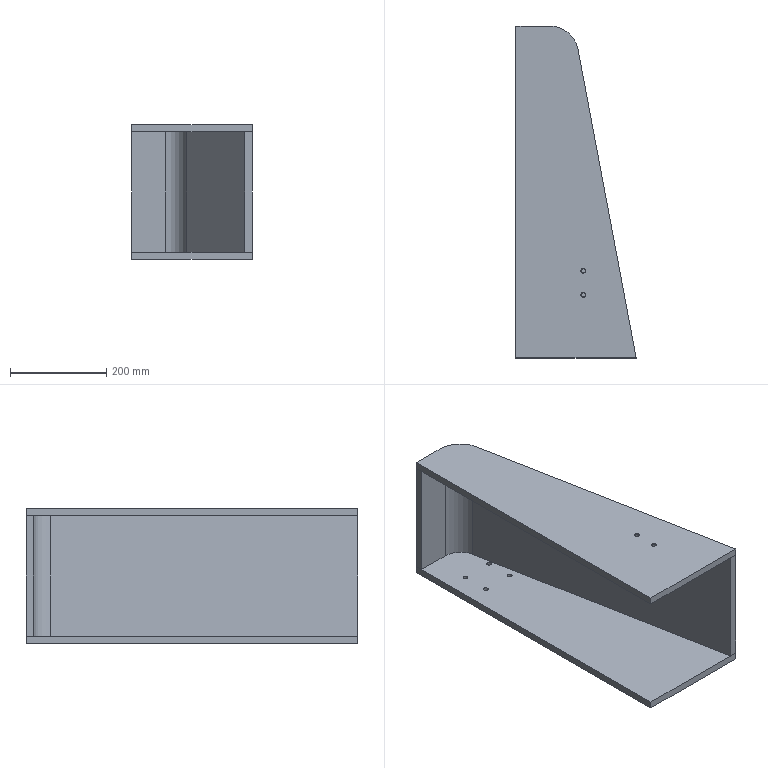Part | SolidWorks | features 3DProfileFeature 2, HoleWzd 2, ICE 2, Extrusion 1 | 3 solids | 48 faces | box 250 x 690 x 280 mm | volume 6785212 mm3 | plane 20 | cylinder 16 | cone 12 | commonest cylinder face diameters 10.2 x8 8.5 x4 120 x3 90 x1
STEP:
#1=CARTESIAN_POINT('',(129.211,641.109,0.));
#2=VERTEX_POINT('',#1);
#3=CARTESIAN_POINT('',(250.,0.,0.));
#4=VERTEX_POINT('',#3);
#5=CARTESIAN_POINT('',(129.211,641.109,0.));
#6=DIRECTION('',(0.1851,-0.9827,0.));
#7=VECTOR('',#6,1000.);
#8=LINE('',#5,#7);
#9=EDGE_CURVE('',#2,#4,#8,.T.);
#10=ORIENTED_EDGE('',*,*,#9,.T.);
#11=CARTESIAN_POINT('',(250.,0.,-250.));
#12=VERTEX_POINT('',#11);
#13=CARTESIAN_POINT('',(250.,0.,-250.));
#14=DIRECTION('',(0.,0.,1.));
#15=VECTOR('',#14,1000.);
#16=LINE('',#13,#15);
#17=EDGE_CURVE('',#12,#4,#16,.T.);
#18=ORIENTED_EDGE('',*,*,#17,.F.);
#19=CARTESIAN_POINT('',(129.211,641.109,-250.));
#20=VERTEX_POINT('',#19);
#21=CARTESIAN_POINT('',(129.211,641.109,-250.));
#22=DIRECTION('',(0.1851,-0.9827,0.));
#23=VECTOR('',#22,1000.);
#24=LINE('',#21,#23);
#25=EDGE_CURVE('',#20,#12,#24,.T.);
#26=ORIENTED_EDGE('',*,*,#25,.F.);
#27=CARTESIAN_POINT('',(129.211,641.109,-250.));
#28=DIRECTION('',(0.,0.,1.));
#29=VECTOR('',#28,1000.);
#30=LINE('',#27,#29);
#31=EDGE_CURVE('',#20,#2,#30,.T.);
#32=ORIENTED_EDGE('',*,*,#31,.T.);
#33=EDGE_LOOP('',(#10,#18,#26,#32));
#34=FACE_OUTER_BOUND('',#33,.T.);
#35=CARTESIAN_POINT('',(129.211,641.109,-250.));
#36=DIRECTION('',(-0.9827,-0.1851,0.));
#37=DIRECTION('',(0.1851,-0.9827,0.));
#38=AXIS2_PLACEMENT_3D('',#35,#36,#37);
#39=PLANE('',#38);
#40=ADVANCED_FACE('',(#34),#39,.F.);
#41=CARTESIAN_POINT('',(234.736,0.,0.));
#42=VERTEX_POINT('',#41);
#43=CARTESIAN_POINT('',(250.,0.,0.));
#44=DIRECTION('',(-1.,0.,0.));
#45=VECTOR('',#44,1000.);
#46=LINE('',#43,#45);
#47=EDGE_CURVE('',#4,#42,#46,.T.);
#48=ORIENTED_EDGE('',*,*,#47,.T.);
#49=CARTESIAN_POINT('',(234.736,0.,-250.));
#50=VERTEX_POINT('',#49);
#51=CARTESIAN_POINT('',(234.736,0.,-250.));
#52=DIRECTION('',(0.,0.,1.));
#53=VECTOR('',#52,1000.);
#54=LINE('',#51,#53);
#55=EDGE_CURVE('',#50,#42,#54,.T.);
#56=ORIENTED_EDGE('',*,*,#55,.F.);
#57=CARTESIAN_POINT('',(250.,0.,-250.));
#58=DIRECTION('',(-1.,0.,0.));
#59=VECTOR('',#58,1000.);
#60=LINE('',#57,#59);
#61=EDGE_CURVE('',#12,#50,#60,.T.);
#62=ORIENTED_EDGE('',*,*,#61,.F.);
#63=ORIENTED_EDGE('',*,*,#17,.T.);
#64=EDGE_LOOP('',(#48,#56,#62,#63));
#65=FACE_OUTER_BOUND('',#64,.T.);
#66=CARTESIAN_POINT('',(250.,0.,-250.));
#67=DIRECTION('',(0.,1.,0.));
#68=DIRECTION('',(-1.,0.,0.));
#69=AXIS2_PLACEMENT_3D('',#66,#67,#68);
#70=PLANE('',#69);
#71=ADVANCED_FACE('',(#65),#70,.F.);
#72=CARTESIAN_POINT('',(114.471,638.332,0.));
#73=VERTEX_POINT('',#72);
#74=CARTESIAN_POINT('',(114.471,638.332,0.));
#75=DIRECTION('',(-0.1851,0.9827,0.));
#76=VECTOR('',#75,1000.);
#77=LINE('',#74,#76);
#78=EDGE_CURVE('',#42,#73,#77,.T.);
#79=ORIENTED_EDGE('',*,*,#78,.T.);
#80=CARTESIAN_POINT('',(114.471,638.332,-250.));
#81=VERTEX_POINT('',#80);
#82=CARTESIAN_POINT('',(114.471,638.332,-250.));
#83=DIRECTION('',(0.,0.,1.));
#84=VECTOR('',#83,1000.);
#85=LINE('',#82,#84);
#86=EDGE_CURVE('',#81,#73,#85,.T.);
#87=ORIENTED_EDGE('',*,*,#86,.F.);
#88=CARTESIAN_POINT('',(114.471,638.332,-250.));
#89=DIRECTION('',(-0.1851,0.9827,0.));
#90=VECTOR('',#89,1000.);
#91=LINE('',#88,#90);
#92=EDGE_CURVE('',#50,#81,#91,.T.);
#93=ORIENTED_EDGE('',*,*,#92,.F.);
#94=ORIENTED_EDGE('',*,*,#55,.T.);
#95=EDGE_LOOP('',(#79,#87,#93,#94));
#96=FACE_OUTER_BOUND('',#95,.T.);
#97=CARTESIAN_POINT('',(114.471,638.332,-250.));
#98=DIRECTION('',(0.9827,0.1851,0.));
#99=DIRECTION('',(-0.1851,0.9827,0.));
#100=AXIS2_PLACEMENT_3D('',#97,#98,#99);
#101=PLANE('',#100);
#102=ADVANCED_FACE('',(#96),#101,.F.);
#103=CARTESIAN_POINT('',(70.249,675.,0.));
#104=VERTEX_POINT('',#103);
#105=CARTESIAN_POINT('',(70.249,630.,0.));
#106=DIRECTION('',(0.,0.,1.));
#107=DIRECTION('',(-1.,0.,0.));
#108=AXIS2_PLACEMENT_3D('',#105,#106,#107);
#109=CIRCLE('',#108,45.);
#110=EDGE_CURVE('',#73,#104,#109,.T.);
#111=ORIENTED_EDGE('',*,*,#110,.T.);
#112=CARTESIAN_POINT('',(70.249,675.,-250.));
#113=VERTEX_POINT('',#112);
#114=CARTESIAN_POINT('',(70.249,675.,-250.));
#115=DIRECTION('',(0.,0.,1.));
#116=VECTOR('',#115,1000.);
#117=LINE('',#114,#116);
#118=EDGE_CURVE('',#113,#104,#117,.T.);
#119=ORIENTED_EDGE('',*,*,#118,.F.);
#120=CARTESIAN_POINT('',(70.249,630.,-250.));
#121=DIRECTION('',(0.,0.,1.));
#122=DIRECTION('',(-1.,0.,0.));
#123=AXIS2_PLACEMENT_3D('',#120,#121,#122);
#124=CIRCLE('',#123,45.);
#125=EDGE_CURVE('',#81,#113,#124,.T.);
#126=ORIENTED_EDGE('',*,*,#125,.F.);
#127=ORIENTED_EDGE('',*,*,#86,.T.);
#128=EDGE_LOOP('',(#111,#119,#126,#127));
#129=FACE_OUTER_BOUND('',#128,.T.);
#130=CARTESIAN_POINT('',(70.249,630.,-250.));
#131=DIRECTION('',(0.,0.,1.));
#132=DIRECTION('',(1.,0.,0.));
#133=AXIS2_PLACEMENT_3D('',#130,#131,#132);
#134=CYLINDRICAL_SURFACE('',#133,45.);
#135=ADVANCED_FACE('',(#129),#134,.F.);
#136=CARTESIAN_POINT('',(0.,675.,0.));
#137=VERTEX_POINT('',#136);
#138=CARTESIAN_POINT('',(0.,675.,0.));
#139=DIRECTION('',(-1.,0.,0.));
#140=VECTOR('',#139,1000.);
#141=LINE('',#138,#140);
#142=EDGE_CURVE('',#104,#137,#141,.T.);
#143=ORIENTED_EDGE('',*,*,#142,.T.);
#144=CARTESIAN_POINT('',(0.,675.,-250.));
#145=VERTEX_POINT('',#144);
#146=CARTESIAN_POINT('',(0.,675.,-250.));
#147=DIRECTION('',(0.,0.,1.));
#148=VECTOR('',#147,1000.);
#149=LINE('',#146,#148);
#150=EDGE_CURVE('',#145,#137,#149,.T.);
#151=ORIENTED_EDGE('',*,*,#150,.F.);
#152=CARTESIAN_POINT('',(0.,675.,-250.));
#153=DIRECTION('',(-1.,0.,0.));
#154=VECTOR('',#153,1000.);
#155=LINE('',#152,#154);
#156=EDGE_CURVE('',#113,#145,#155,.T.);
#157=ORIENTED_EDGE('',*,*,#156,.F.);
#158=ORIENTED_EDGE('',*,*,#118,.T.);
#159=EDGE_LOOP('',(#143,#151,#157,#158));
#160=FACE_OUTER_BOUND('',#159,.T.);
#161=CARTESIAN_POINT('',(0.,675.,-250.));
#162=DIRECTION('',(0.,1.,0.));
#163=DIRECTION('',(0.,0.,1.));
#164=AXIS2_PLACEMENT_3D('',#161,#162,#163);
#165=PLANE('',#164);
#166=ADVANCED_FACE('',(#160),#165,.F.);
#167=CARTESIAN_POINT('',(0.,690.,0.));
#168=VERTEX_POINT('',#167);
#169=CARTESIAN_POINT('',(0.,690.,0.));
#170=DIRECTION('',(0.,1.,0.));
#171=VECTOR('',#170,1000.);
#172=LINE('',#169,#171);
#173=EDGE_CURVE('',#137,#168,#172,.T.);
#174=ORIENTED_EDGE('',*,*,#173,.T.);
#175=CARTESIAN_POINT('',(0.,690.,-250.));
#176=VERTEX_POINT('',#175);
#177=CARTESIAN_POINT('',(0.,690.,-250.));
#178=DIRECTION('',(0.,0.,1.));
#179=VECTOR('',#178,1000.);
#180=LINE('',#177,#179);
#181=EDGE_CURVE('',#176,#168,#180,.T.);
#182=ORIENTED_EDGE('',*,*,#181,.F.);
#183=CARTESIAN_POINT('',(0.,690.,-250.));
#184=DIRECTION('',(0.,1.,0.));
#185=VECTOR('',#184,1000.);
#186=LINE('',#183,#185);
#187=EDGE_CURVE('',#145,#176,#186,.T.);
#188=ORIENTED_EDGE('',*,*,#187,.F.);
#189=ORIENTED_EDGE('',*,*,#150,.T.);
#190=EDGE_LOOP('',(#174,#182,#188,#189));
#191=FACE_OUTER_BOUND('',#190,.T.);
#192=CARTESIAN_POINT('',(0.,690.,-250.));
#193=DIRECTION('',(1.,0.,0.));
#194=DIRECTION('',(0.,1.,0.));
#195=AXIS2_PLACEMENT_3D('',#192,#193,#194);
#196=PLANE('',#195);
#197=ADVANCED_FACE('',(#191),#196,.F.);
#198=CARTESIAN_POINT('',(70.249,690.,0.));
#199=VERTEX_POINT('',#198);
#200=CARTESIAN_POINT('',(0.,690.,0.));
#201=DIRECTION('',(1.,0.,0.));
#202=VECTOR('',#201,1000.);
#203=LINE('',#200,#202);
#204=EDGE_CURVE('',#168,#199,#203,.T.);
#205=ORIENTED_EDGE('',*,*,#204,.T.);
#206=CARTESIAN_POINT('',(70.249,690.,-250.));
#207=VERTEX_POINT('',#206);
#208=CARTESIAN_POINT('',(70.249,690.,-250.));
#209=DIRECTION('',(0.,0.,1.));
#210=VECTOR('',#209,1000.);
#211=LINE('',#208,#210);
#212=EDGE_CURVE('',#207,#199,#211,.T.);
#213=ORIENTED_EDGE('',*,*,#212,.F.);
#214=CARTESIAN_POINT('',(0.,690.,-250.));
#215=DIRECTION('',(1.,0.,0.));
#216=VECTOR('',#215,1000.);
#217=LINE('',#214,#216);
#218=EDGE_CURVE('',#176,#207,#217,.T.);
#219=ORIENTED_EDGE('',*,*,#218,.F.);
#220=ORIENTED_EDGE('',*,*,#181,.T.);
#221=EDGE_LOOP('',(#205,#213,#219,#220));
#222=FACE_OUTER_BOUND('',#221,.T.);
#223=CARTESIAN_POINT('',(0.,690.,-250.));
#224=DIRECTION('',(0.,-1.,0.));
#225=DIRECTION('',(1.,0.,0.));
#226=AXIS2_PLACEMENT_3D('',#223,#224,#225);
#227=PLANE('',#226);
#228=ADVANCED_FACE('',(#222),#227,.F.);
#229=CARTESIAN_POINT('',(70.249,630.,0.));
#230=DIRECTION('',(0.,0.,-1.));
#231=DIRECTION('',(-1.,0.,0.));
#232=AXIS2_PLACEMENT_3D('',#229,#230,#231);
#233=CIRCLE('',#232,60.);
#234=EDGE_CURVE('',#199,#2,#233,.T.);
#235=ORIENTED_EDGE('',*,*,#234,.T.);
#236=ORIENTED_EDGE('',*,*,#31,.F.);
#237=CARTESIAN_POINT('',(70.249,630.,-250.));
#238=DIRECTION('',(0.,0.,-1.));
#239=DIRECTION('',(-1.,0.,0.));
#240=AXIS2_PLACEMENT_3D('',#237,#238,#239);
#241=CIRCLE('',#240,60.);
#242=EDGE_CURVE('',#207,#20,#241,.T.);
#243=ORIENTED_EDGE('',*,*,#242,.F.);
#244=ORIENTED_EDGE('',*,*,#212,.T.);
#245=EDGE_LOOP('',(#235,#236,#243,#244));
#246=FACE_OUTER_BOUND('',#245,.T.);
#247=CARTESIAN_POINT('',(70.249,630.,-250.));
#248=DIRECTION('',(0.,0.,1.));
#249=DIRECTION('',(1.,0.,0.));
#250=AXIS2_PLACEMENT_3D('',#247,#248,#249);
#251=CYLINDRICAL_SURFACE('',#250,60.);
#252=ADVANCED_FACE('',(#246),#251,.T.);
#253=ORIENTED_EDGE('',*,*,#25,.T.);
#254=ORIENTED_EDGE('',*,*,#61,.T.);
#255=ORIENTED_EDGE('',*,*,#92,.T.);
#256=ORIENTED_EDGE('',*,*,#125,.T.);
#257=ORIENTED_EDGE('',*,*,#156,.T.);
#258=ORIENTED_EDGE('',*,*,#187,.T.);
#259=ORIENTED_EDGE('',*,*,#218,.T.);
#260=ORIENTED_EDGE('',*,*,#242,.T.);
#261=EDGE_LOOP('',(#253,#254,#255,#256,#257,#258,#259,#260));
#262=FACE_OUTER_BOUND('',#261,.T.);
#263=CARTESIAN_POINT('',(70.249,630.,-250.));
#264=DIRECTION('',(0.,0.,-1.));
#265=DIRECTION('',(-1.,0.,0.));
#266=AXIS2_PLACEMENT_3D('',#263,#264,#265);
#267=PLANE('',#266);
#268=ADVANCED_FACE('',(#262),#267,.T.);
#269=ORIENTED_EDGE('',*,*,#9,.F.);
#270=ORIENTED_EDGE('',*,*,#234,.F.);
#271=ORIENTED_EDGE('',*,*,#204,.F.);
#272=ORIENTED_EDGE('',*,*,#173,.F.);
#273=ORIENTED_EDGE('',*,*,#142,.F.);
#274=ORIENTED_EDGE('',*,*,#110,.F.);
#275=ORIENTED_EDGE('',*,*,#78,.F.);
#276=ORIENTED_EDGE('',*,*,#47,.F.);
#277=EDGE_LOOP('',(#269,#270,#271,#272,#273,#274,#275,#276));
#278=FACE_OUTER_BOUND('',#277,.T.);
#279=CARTESIAN_POINT('',(70.249,630.,0.));
#280=DIRECTION('',(0.,0.,-1.));
#281=DIRECTION('',(-1.,0.,0.));
#282=AXIS2_PLACEMENT_3D('',#279,#280,#281);
#283=PLANE('',#282);
#284=ADVANCED_FACE('',(#278),#283,.F.);
#285=CLOSED_SHELL('',(#40,#71,#102,#135,#166,#197,#228,#252,#268,#284));
#286=MANIFOLD_SOLID_BREP('',#285);
#287=CARTESIAN_POINT('',(135.75,181.,14.225));
#288=VERTEX_POINT('',#287);
#289=CARTESIAN_POINT('',(144.25,181.,14.225));
#290=VERTEX_POINT('',#289);
#291=CARTESIAN_POINT('',(140.,181.,14.225));
#292=DIRECTION('',(0.,0.,1.));
#293=DIRECTION('',(1.,0.,0.));
#294=AXIS2_PLACEMENT_3D('',#291,#292,#293);
#295=CIRCLE('',#294,4.25);
#296=EDGE_CURVE('',#288,#290,#295,.T.);
#297=ORIENTED_EDGE('',*,*,#296,.F.);
#298=CARTESIAN_POINT('',(134.975,181.,15.));
#299=VERTEX_POINT('',#298);
#300=CARTESIAN_POINT('',(134.975,181.,15.));
#301=DIRECTION('',(-0.7071,0.,0.7071));
#302=VECTOR('',#301,1000.);
#303=LINE('',#300,#302);
#304=EDGE_CURVE('',#288,#299,#303,.T.);
#305=ORIENTED_EDGE('',*,*,#304,.T.);
#306=CARTESIAN_POINT('',(145.025,181.,15.));
#307=VERTEX_POINT('',#306);
#308=CARTESIAN_POINT('',(140.,181.,15.));
#309=DIRECTION('',(0.,0.,1.));
#310=DIRECTION('',(1.,0.,0.));
#311=AXIS2_PLACEMENT_3D('',#308,#309,#310);
#312=CIRCLE('',#311,5.025);
#313=EDGE_CURVE('',#299,#307,#312,.T.);
#314=ORIENTED_EDGE('',*,*,#313,.T.);
#315=CARTESIAN_POINT('',(145.025,181.,15.));
#316=DIRECTION('',(0.7071,0.,0.7071));
#317=VECTOR('',#316,1000.);
#318=LINE('',#315,#317);
#319=EDGE_CURVE('',#290,#307,#318,.T.);
#320=ORIENTED_EDGE('',*,*,#319,.F.);
#321=EDGE_LOOP('',(#297,#305,#314,#320));
#322=FACE_OUTER_BOUND('',#321,.T.);
#323=CARTESIAN_POINT('',(140.,181.,15.));
#324=DIRECTION('',(0.,0.,1.));
#325=DIRECTION('',(1.,0.,0.));
#326=AXIS2_PLACEMENT_3D('',#323,#324,#325);
#327=CONICAL_SURFACE('',#326,5.025,0.7854);
#328=ADVANCED_FACE('',(#322),#327,.F.);
#329=CARTESIAN_POINT('',(135.75,181.,0.));
#330=VERTEX_POINT('',#329);
#331=CARTESIAN_POINT('',(144.25,181.,0.));
#332=VERTEX_POINT('',#331);
#333=CARTESIAN_POINT('',(140.,181.,0.));
#334=DIRECTION('',(0.,0.,1.));
#335=DIRECTION('',(1.,0.,0.));
#336=AXIS2_PLACEMENT_3D('',#333,#334,#335);
#337=CIRCLE('',#336,4.25);
#338=EDGE_CURVE('',#330,#332,#337,.T.);
#339=ORIENTED_EDGE('',*,*,#338,.F.);
#340=CARTESIAN_POINT('',(135.75,181.,15.));
#341=DIRECTION('',(0.,0.,1.));
#342=VECTOR('',#341,1000.);
#343=LINE('',#340,#342);
#344=EDGE_CURVE('',#330,#288,#343,.T.);
#345=ORIENTED_EDGE('',*,*,#344,.T.);
#346=ORIENTED_EDGE('',*,*,#296,.T.);
#347=CARTESIAN_POINT('',(144.25,181.,15.));
#348=DIRECTION('',(0.,0.,1.));
#349=VECTOR('',#348,1000.);
#350=LINE('',#347,#349);
#351=EDGE_CURVE('',#332,#290,#350,.T.);
#352=ORIENTED_EDGE('',*,*,#351,.F.);
#353=EDGE_LOOP('',(#339,#345,#346,#352));
#354=FACE_OUTER_BOUND('',#353,.T.);
#355=CARTESIAN_POINT('',(140.,181.,15.));
#356=DIRECTION('',(0.,0.,1.));
#357=DIRECTION('',(1.,0.,0.));
#358=AXIS2_PLACEMENT_3D('',#355,#356,#357);
#359=CYLINDRICAL_SURFACE('',#358,4.25);
#360=ADVANCED_FACE('',(#354),#359,.F.);
#361=CARTESIAN_POINT('',(135.75,131.,14.225));
#362=VERTEX_POINT('',#361);
#363=CARTESIAN_POINT('',(144.25,131.,14.225));
#364=VERTEX_POINT('',#363);
#365=CARTESIAN_POINT('',(140.,131.,14.225));
#366=DIRECTION('',(0.,0.,1.));
#367=DIRECTION('',(1.,0.,0.));
#368=AXIS2_PLACEMENT_3D('',#365,#366,#367);
#369=CIRCLE('',#368,4.25);
#370=EDGE_CURVE('',#362,#364,#369,.T.);
#371=ORIENTED_EDGE('',*,*,#370,.F.);
#372=CARTESIAN_POINT('',(134.975,131.,15.));
#373=VERTEX_POINT('',#372);
#374=CARTESIAN_POINT('',(134.975,131.,15.));
#375=DIRECTION('',(-0.7071,0.,0.7071));
#376=VECTOR('',#375,1000.);
#377=LINE('',#374,#376);
#378=EDGE_CURVE('',#362,#373,#377,.T.);
#379=ORIENTED_EDGE('',*,*,#378,.T.);
#380=CARTESIAN_POINT('',(145.025,131.,15.));
#381=VERTEX_POINT('',#380);
#382=CARTESIAN_POINT('',(140.,131.,15.));
#383=DIRECTION('',(0.,0.,1.));
#384=DIRECTION('',(1.,0.,0.));
#385=AXIS2_PLACEMENT_3D('',#382,#383,#384);
#386=CIRCLE('',#385,5.025);
#387=EDGE_CURVE('',#373,#381,#386,.T.);
#388=ORIENTED_EDGE('',*,*,#387,.T.);
#389=CARTESIAN_POINT('',(145.025,131.,15.));
#390=DIRECTION('',(0.7071,0.,0.7071));
#391=VECTOR('',#390,1000.);
#392=LINE('',#389,#391);
#393=EDGE_CURVE('',#364,#381,#392,.T.);
#394=ORIENTED_EDGE('',*,*,#393,.F.);
#395=EDGE_LOOP('',(#371,#379,#388,#394));
#396=FACE_OUTER_BOUND('',#395,.T.);
#397=CARTESIAN_POINT('',(140.,131.,15.));
#398=DIRECTION('',(0.,0.,1.));
#399=DIRECTION('',(1.,0.,0.));
#400=AXIS2_PLACEMENT_3D('',#397,#398,#399);
#401=CONICAL_SURFACE('',#400,5.025,0.7854);
#402=ADVANCED_FACE('',(#396),#401,.F.);
#403=CARTESIAN_POINT('',(135.75,131.,0.));
#404=VERTEX_POINT('',#403);
#405=CARTESIAN_POINT('',(144.25,131.,0.));
#406=VERTEX_POINT('',#405);
#407=CARTESIAN_POINT('',(140.,131.,0.));
#408=DIRECTION('',(0.,0.,1.));
#409=DIRECTION('',(1.,0.,0.));
#410=AXIS2_PLACEMENT_3D('',#407,#408,#409);
#411=CIRCLE('',#410,4.25);
#412=EDGE_CURVE('',#404,#406,#411,.T.);
#413=ORIENTED_EDGE('',*,*,#412,.F.);
#414=CARTESIAN_POINT('',(135.75,131.,15.));
#415=DIRECTION('',(0.,0.,1.));
#416=VECTOR('',#415,1000.);
#417=LINE('',#414,#416);
#418=EDGE_CURVE('',#404,#362,#417,.T.);
#419=ORIENTED_EDGE('',*,*,#418,.T.);
#420=ORIENTED_EDGE('',*,*,#370,.T.);
#421=CARTESIAN_POINT('',(144.25,131.,15.));
#422=DIRECTION('',(0.,0.,1.));
#423=VECTOR('',#422,1000.);
#424=LINE('',#421,#423);
#425=EDGE_CURVE('',#406,#364,#424,.T.);
#426=ORIENTED_EDGE('',*,*,#425,.F.);
#427=EDGE_LOOP('',(#413,#419,#420,#426));
#428=FACE_OUTER_BOUND('',#427,.T.);
#429=CARTESIAN_POINT('',(140.,131.,15.));
#430=DIRECTION('',(0.,0.,1.));
#431=DIRECTION('',(1.,0.,0.));
#432=AXIS2_PLACEMENT_3D('',#429,#430,#431);
#433=CYLINDRICAL_SURFACE('',#432,4.25);
#434=ADVANCED_FACE('',(#428),#433,.F.);
#435=CARTESIAN_POINT('',(0.,0.,0.));
#436=VERTEX_POINT('',#435);
#437=CARTESIAN_POINT('',(250.,0.,0.));
#438=VERTEX_POINT('',#437);
#439=CARTESIAN_POINT('',(250.,0.,0.));
#440=DIRECTION('',(1.,0.,0.));
#441=VECTOR('',#440,1000.);
#442=LINE('',#439,#441);
#443=EDGE_CURVE('',#436,#438,#442,.T.);
#444=ORIENTED_EDGE('',*,*,#443,.T.);
#445=CARTESIAN_POINT('',(250.,0.,15.));
#446=VERTEX_POINT('',#445);
#447=CARTESIAN_POINT('',(250.,0.,15.));
#448=DIRECTION('',(0.,0.,-1.));
#449=VECTOR('',#448,1000.);
#450=LINE('',#447,#449);
#451=EDGE_CURVE('',#446,#438,#450,.T.);
#452=ORIENTED_EDGE('',*,*,#451,.F.);
#453=CARTESIAN_POINT('',(0.,0.,15.));
#454=VERTEX_POINT('',#453);
#455=CARTESIAN_POINT('',(250.,0.,15.));
#456=DIRECTION('',(1.,0.,0.));
#457=VECTOR('',#456,1000.);
#458=LINE('',#455,#457);
#459=EDGE_CURVE('',#454,#446,#458,.T.);
#460=ORIENTED_EDGE('',*,*,#459,.F.);
#461=CARTESIAN_POINT('',(0.,0.,15.));
#462=DIRECTION('',(0.,0.,-1.));
#463=VECTOR('',#462,1000.);
#464=LINE('',#461,#463);
#465=EDGE_CURVE('',#454,#436,#464,.T.);
#466=ORIENTED_EDGE('',*,*,#465,.T.);
#467=EDGE_LOOP('',(#444,#452,#460,#466));
#468=FACE_OUTER_BOUND('',#467,.T.);
#469=CARTESIAN_POINT('',(250.,0.,15.));
#470=DIRECTION('',(0.,1.,0.));
#471=DIRECTION('',(-1.,0.,0.));
#472=AXIS2_PLACEMENT_3D('',#469,#470,#471);
#473=PLANE('',#472);
#474=ADVANCED_FACE('',(#468),#473,.F.);
#475=CARTESIAN_POINT('',(129.211,641.109,0.));
#476=VERTEX_POINT('',#475);
#477=CARTESIAN_POINT('',(129.211,641.109,0.));
#478=DIRECTION('',(-0.1851,0.9827,0.));
#479=VECTOR('',#478,1000.);
#480=LINE('',#477,#479);
#481=EDGE_CURVE('',#438,#476,#480,.T.);
#482=ORIENTED_EDGE('',*,*,#481,.T.);
#483=CARTESIAN_POINT('',(129.211,641.109,15.));
#484=VERTEX_POINT('',#483);
#485=CARTESIAN_POINT('',(129.211,641.109,15.));
#486=DIRECTION('',(0.,0.,-1.));
#487=VECTOR('',#486,1000.);
#488=LINE('',#485,#487);
#489=EDGE_CURVE('',#484,#476,#488,.T.);
#490=ORIENTED_EDGE('',*,*,#489,.F.);
#491=CARTESIAN_POINT('',(129.211,641.109,15.));
#492=DIRECTION('',(-0.1851,0.9827,0.));
#493=VECTOR('',#492,1000.);
#494=LINE('',#491,#493);
#495=EDGE_CURVE('',#446,#484,#494,.T.);
#496=ORIENTED_EDGE('',*,*,#495,.F.);
#497=ORIENTED_EDGE('',*,*,#451,.T.);
#498=EDGE_LOOP('',(#482,#490,#496,#497));
#499=FACE_OUTER_BOUND('',#498,.T.);
#500=CARTESIAN_POINT('',(129.211,641.109,15.));
#501=DIRECTION('',(-0.9827,-0.1851,0.));
#502=DIRECTION('',(0.1851,-0.9827,0.));
#503=AXIS2_PLACEMENT_3D('',#500,#501,#502);
#504=PLANE('',#503);
#505=ADVANCED_FACE('',(#499),#504,.F.);
#506=CARTESIAN_POINT('',(70.249,690.,0.));
#507=VERTEX_POINT('',#506);
#508=CARTESIAN_POINT('',(70.249,630.,0.));
#509=DIRECTION('',(0.,0.,1.));
#510=DIRECTION('',(1.,0.,0.));
#511=AXIS2_PLACEMENT_3D('',#508,#509,#510);
#512=CIRCLE('',#511,60.);
#513=EDGE_CURVE('',#476,#507,#512,.T.);
#514=ORIENTED_EDGE('',*,*,#513,.T.);
#515=CARTESIAN_POINT('',(70.249,690.,15.));
#516=VERTEX_POINT('',#515);
#517=CARTESIAN_POINT('',(70.249,690.,15.));
#518=DIRECTION('',(0.,0.,-1.));
#519=VECTOR('',#518,1000.);
#520=LINE('',#517,#519);
#521=EDGE_CURVE('',#516,#507,#520,.T.);
#522=ORIENTED_EDGE('',*,*,#521,.F.);
#523=CARTESIAN_POINT('',(70.249,630.,15.));
#524=DIRECTION('',(0.,0.,1.));
#525=DIRECTION('',(1.,0.,0.));
#526=AXIS2_PLACEMENT_3D('',#523,#524,#525);
#527=CIRCLE('',#526,60.);
#528=EDGE_CURVE('',#484,#516,#527,.T.);
#529=ORIENTED_EDGE('',*,*,#528,.F.);
#530=ORIENTED_EDGE('',*,*,#489,.T.);
#531=EDGE_LOOP('',(#514,#522,#529,#530));
#532=FACE_OUTER_BOUND('',#531,.T.);
#533=CARTESIAN_POINT('',(70.249,630.,15.));
#534=DIRECTION('',(0.,0.,-1.));
#535=DIRECTION('',(-1.,0.,0.));
#536=AXIS2_PLACEMENT_3D('',#533,#534,#535);
#537=CYLINDRICAL_SURFACE('',#536,60.);
#538=ADVANCED_FACE('',(#532),#537,.T.);
#539=CARTESIAN_POINT('',(0.,690.,0.));
#540=VERTEX_POINT('',#539);
#541=CARTESIAN_POINT('',(0.,690.,0.));
#542=DIRECTION('',(-1.,0.,0.));
#543=VECTOR('',#542,1000.);
#544=LINE('',#541,#543);
#545=EDGE_CURVE('',#507,#540,#544,.T.);
#546=ORIENTED_EDGE('',*,*,#545,.T.);
#547=CARTESIAN_POINT('',(0.,690.,15.));
#548=VERTEX_POINT('',#547);
#549=CARTESIAN_POINT('',(0.,690.,15.));
#550=DIRECTION('',(0.,0.,-1.));
#551=VECTOR('',#550,1000.);
#552=LINE('',#549,#551);
#553=EDGE_CURVE('',#548,#540,#552,.T.);
#554=ORIENTED_EDGE('',*,*,#553,.F.);
#555=CARTESIAN_POINT('',(0.,690.,15.));
#556=DIRECTION('',(-1.,0.,0.));
#557=VECTOR('',#556,1000.);
#558=LINE('',#555,#557);
#559=EDGE_CURVE('',#516,#548,#558,.T.);
#560=ORIENTED_EDGE('',*,*,#559,.F.);
#561=ORIENTED_EDGE('',*,*,#521,.T.);
#562=EDGE_LOOP('',(#546,#554,#560,#561));
#563=FACE_OUTER_BOUND('',#562,.T.);
#564=CARTESIAN_POINT('',(0.,690.,15.));
#565=DIRECTION('',(0.,-1.,0.));
#566=DIRECTION('',(1.,0.,0.));
#567=AXIS2_PLACEMENT_3D('',#564,#565,#566);
#568=PLANE('',#567);
#569=ADVANCED_FACE('',(#563),#568,.F.);
#570=CARTESIAN_POINT('',(0.,0.,0.));
#571=DIRECTION('',(0.,-1.,0.));
#572=VECTOR('',#571,1000.);
#573=LINE('',#570,#572);
#574=EDGE_CURVE('',#540,#436,#573,.T.);
#575=ORIENTED_EDGE('',*,*,#574,.T.);
#576=ORIENTED_EDGE('',*,*,#465,.F.);
#577=CARTESIAN_POINT('',(0.,0.,15.));
#578=DIRECTION('',(0.,-1.,0.));
#579=VECTOR('',#578,1000.);
#580=LINE('',#577,#579);
#581=EDGE_CURVE('',#548,#454,#580,.T.);
#582=ORIENTED_EDGE('',*,*,#581,.F.);
#583=ORIENTED_EDGE('',*,*,#553,.T.);
#584=EDGE_LOOP('',(#575,#576,#582,#583));
#585=FACE_OUTER_BOUND('',#584,.T.);
#586=CARTESIAN_POINT('',(0.,0.,15.));
#587=DIRECTION('',(1.,0.,0.));
#588=DIRECTION('',(0.,0.,-1.));
#589=AXIS2_PLACEMENT_3D('',#586,#587,#588);
#590=PLANE('',#589);
#591=ADVANCED_FACE('',(#585),#590,.F.);
#592=CARTESIAN_POINT('',(140.,181.,15.));
#593=DIRECTION('',(0.,0.,1.));
#594=DIRECTION('',(1.,0.,0.));
#595=AXIS2_PLACEMENT_3D('',#592,#593,#594);
#596=CIRCLE('',#595,5.025);
#597=EDGE_CURVE('',#307,#299,#596,.T.);
#598=ORIENTED_EDGE('',*,*,#597,.F.);
#599=ORIENTED_EDGE('',*,*,#313,.F.);
#600=EDGE_LOOP('',(#598,#599));
#601=FACE_BOUND('',#600,.T.);
#602=CARTESIAN_POINT('',(140.,131.,15.));
#603=DIRECTION('',(0.,0.,1.));
#604=DIRECTION('',(1.,0.,0.));
#605=AXIS2_PLACEMENT_3D('',#602,#603,#604);
#606=CIRCLE('',#605,5.025);
#607=EDGE_CURVE('',#381,#373,#606,.T.);
#608=ORIENTED_EDGE('',*,*,#607,.F.);
#609=ORIENTED_EDGE('',*,*,#387,.F.);
#610=EDGE_LOOP('',(#608,#609));
#611=FACE_BOUND('',#610,.T.);
#612=ORIENTED_EDGE('',*,*,#459,.T.);
#613=ORIENTED_EDGE('',*,*,#495,.T.);
#614=ORIENTED_EDGE('',*,*,#528,.T.);
#615=ORIENTED_EDGE('',*,*,#559,.T.);
#616=ORIENTED_EDGE('',*,*,#581,.T.);
#617=EDGE_LOOP('',(#612,#613,#614,#615,#616));
#618=FACE_OUTER_BOUND('',#617,.T.);
#619=CARTESIAN_POINT('',(70.249,630.,15.));
#620=DIRECTION('',(0.,0.,1.));
#621=DIRECTION('',(1.,0.,0.));
#622=AXIS2_PLACEMENT_3D('',#619,#620,#621);
#623=PLANE('',#622);
#624=ADVANCED_FACE('',(#601,#611,#618),#623,.T.);
#625=CARTESIAN_POINT('',(140.,181.,0.));
#626=DIRECTION('',(0.,0.,1.));
#627=DIRECTION('',(1.,0.,0.));
#628=AXIS2_PLACEMENT_3D('',#625,#626,#627);
#629=CIRCLE('',#628,4.25);
#630=EDGE_CURVE('',#332,#330,#629,.T.);
#631=ORIENTED_EDGE('',*,*,#630,.T.);
#632=ORIENTED_EDGE('',*,*,#338,.T.);
#633=EDGE_LOOP('',(#631,#632));
#634=FACE_BOUND('',#633,.T.);
#635=CARTESIAN_POINT('',(140.,131.,0.));
#636=DIRECTION('',(0.,0.,1.));
#637=DIRECTION('',(1.,0.,0.));
#638=AXIS2_PLACEMENT_3D('',#635,#636,#637);
#639=CIRCLE('',#638,4.25);
#640=EDGE_CURVE('',#406,#404,#639,.T.);
#641=ORIENTED_EDGE('',*,*,#640,.T.);
#642=ORIENTED_EDGE('',*,*,#412,.T.);
#643=EDGE_LOOP('',(#641,#642));
#644=FACE_BOUND('',#643,.T.);
#645=ORIENTED_EDGE('',*,*,#443,.F.);
#646=ORIENTED_EDGE('',*,*,#574,.F.);
#647=ORIENTED_EDGE('',*,*,#545,.F.);
#648=ORIENTED_EDGE('',*,*,#513,.F.);
#649=ORIENTED_EDGE('',*,*,#481,.F.);
#650=EDGE_LOOP('',(#645,#646,#647,#648,#649));
#651=FACE_OUTER_BOUND('',#650,.T.);
#652=CARTESIAN_POINT('',(70.249,630.,0.));
#653=DIRECTION('',(0.,0.,1.));
#654=DIRECTION('',(1.,0.,0.));
#655=AXIS2_PLACEMENT_3D('',#652,#653,#654);
#656=PLANE('',#655);
#657=ADVANCED_FACE('',(#634,#644,#651),#656,.F.);
#658=ORIENTED_EDGE('',*,*,#418,.F.);
#659=ORIENTED_EDGE('',*,*,#640,.F.);
#660=ORIENTED_EDGE('',*,*,#425,.T.);
#661=CARTESIAN_POINT('',(140.,131.,14.225));
#662=DIRECTION('',(0.,0.,1.));
#663=DIRECTION('',(1.,0.,0.));
#664=AXIS2_PLACEMENT_3D('',#661,#662,#663);
#665=CIRCLE('',#664,4.25);
#666=EDGE_CURVE('',#364,#362,#665,.T.);
#667=ORIENTED_EDGE('',*,*,#666,.T.);
#668=EDGE_LOOP('',(#658,#659,#660,#667));
#669=FACE_OUTER_BOUND('',#668,.T.);
#670=CARTESIAN_POINT('',(140.,131.,15.));
#671=DIRECTION('',(0.,0.,1.));
#672=DIRECTION('',(1.,0.,0.));
#673=AXIS2_PLACEMENT_3D('',#670,#671,#672);
#674=CYLINDRICAL_SURFACE('',#673,4.25);
#675=ADVANCED_FACE('',(#669),#674,.F.);
#676=ORIENTED_EDGE('',*,*,#378,.F.);
#677=ORIENTED_EDGE('',*,*,#666,.F.);
#678=ORIENTED_EDGE('',*,*,#393,.T.);
#679=ORIENTED_EDGE('',*,*,#607,.T.);
#680=EDGE_LOOP('',(#676,#677,#678,#679));
#681=FACE_OUTER_BOUND('',#680,.T.);
#682=CARTESIAN_POINT('',(140.,131.,15.));
#683=DIRECTION('',(0.,0.,1.));
#684=DIRECTION('',(1.,0.,0.));
#685=AXIS2_PLACEMENT_3D('',#682,#683,#684);
#686=CONICAL_SURFACE('',#685,5.025,0.7854);
#687=ADVANCED_FACE('',(#681),#686,.F.);
#688=ORIENTED_EDGE('',*,*,#344,.F.);
#689=ORIENTED_EDGE('',*,*,#630,.F.);
#690=ORIENTED_EDGE('',*,*,#351,.T.);
#691=CARTESIAN_POINT('',(140.,181.,14.225));
#692=DIRECTION('',(0.,0.,1.));
#693=DIRECTION('',(1.,0.,0.));
#694=AXIS2_PLACEMENT_3D('',#691,#692,#693);
#695=CIRCLE('',#694,4.25);
#696=EDGE_CURVE('',#290,#288,#695,.T.);
#697=ORIENTED_EDGE('',*,*,#696,.T.);
#698=EDGE_LOOP('',(#688,#689,#690,#697));
#699=FACE_OUTER_BOUND('',#698,.T.);
#700=CARTESIAN_POINT('',(140.,181.,15.));
#701=DIRECTION('',(0.,0.,1.));
#702=DIRECTION('',(1.,0.,0.));
#703=AXIS2_PLACEMENT_3D('',#700,#701,#702);
#704=CYLINDRICAL_SURFACE('',#703,4.25);
#705=ADVANCED_FACE('',(#699),#704,.F.);
#706=ORIENTED_EDGE('',*,*,#304,.F.);
#707=ORIENTED_EDGE('',*,*,#696,.F.);
#708=ORIENTED_EDGE('',*,*,#319,.T.);
#709=ORIENTED_EDGE('',*,*,#597,.T.);
#710=EDGE_LOOP('',(#706,#707,#708,#709));
#711=FACE_OUTER_BOUND('',#710,.T.);
#712=CARTESIAN_POINT('',(140.,181.,15.));
#713=DIRECTION('',(0.,0.,1.));
#714=DIRECTION('',(1.,0.,0.));
#715=AXIS2_PLACEMENT_3D('',#712,#713,#714);
#716=CONICAL_SURFACE('',#715,5.025,0.7854);
#717=ADVANCED_FACE('',(#711),#716,.F.);
#718=CLOSED_SHELL('',(#328,#360,#402,#434,#474,#505,#538,#569,#591,#624,#657,#675,#687,#705,#717));
#719=MANIFOLD_SOLID_BREP('',#718);
#720=CARTESIAN_POINT('',(50.1,590.,-264.075));
#721=VERTEX_POINT('',#720);
#722=CARTESIAN_POINT('',(39.9,590.,-264.075));
#723=VERTEX_POINT('',#722);
#724=CARTESIAN_POINT('',(45.,590.,-264.075));
#725=DIRECTION('',(0.,0.,-1.));
#726=DIRECTION('',(-1.,0.,0.));
#727=AXIS2_PLACEMENT_3D('',#724,#725,#726);
#728=CIRCLE('',#727,5.1);
#729=EDGE_CURVE('',#721,#723,#728,.T.);
#730=ORIENTED_EDGE('',*,*,#729,.F.);
#731=CARTESIAN_POINT('',(51.025,590.,-265.));
#732=VERTEX_POINT('',#731);
#733=CARTESIAN_POINT('',(51.025,590.,-265.));
#734=DIRECTION('',(0.7071,0.,-0.7071));
#735=VECTOR('',#734,1000.);
#736=LINE('',#733,#735);
#737=EDGE_CURVE('',#721,#732,#736,.T.);
#738=ORIENTED_EDGE('',*,*,#737,.T.);
#739=CARTESIAN_POINT('',(38.975,590.,-265.));
#740=VERTEX_POINT('',#739);
#741=CARTESIAN_POINT('',(45.,590.,-265.));
#742=DIRECTION('',(0.,0.,-1.));
#743=DIRECTION('',(-1.,0.,0.));
#744=AXIS2_PLACEMENT_3D('',#741,#742,#743);
#745=CIRCLE('',#744,6.025);
#746=EDGE_CURVE('',#732,#740,#745,.T.);
#747=ORIENTED_EDGE('',*,*,#746,.T.);
#748=CARTESIAN_POINT('',(38.975,590.,-265.));
#749=DIRECTION('',(-0.7071,0.,-0.7071));
#750=VECTOR('',#749,1000.);
#751=LINE('',#748,#750);
#752=EDGE_CURVE('',#723,#740,#751,.T.);
#753=ORIENTED_EDGE('',*,*,#752,.F.);
#754=EDGE_LOOP('',(#730,#738,#747,#753));
#755=FACE_OUTER_BOUND('',#754,.T.);
#756=CARTESIAN_POINT('',(45.,590.,-265.));
#757=DIRECTION('',(0.,0.,-1.));
#758=DIRECTION('',(-1.,0.,0.));
#759=AXIS2_PLACEMENT_3D('',#756,#757,#758);
#760=CONICAL_SURFACE('',#759,6.025,0.7854);
#761=ADVANCED_FACE('',(#755),#760,.F.);
#762=CARTESIAN_POINT('',(50.1,590.,-250.));
#763=VERTEX_POINT('',#762);
#764=CARTESIAN_POINT('',(39.9,590.,-250.));
#765=VERTEX_POINT('',#764);
#766=CARTESIAN_POINT('',(45.,590.,-250.));
#767=DIRECTION('',(0.,0.,-1.));
#768=DIRECTION('',(-1.,0.,0.));
#769=AXIS2_PLACEMENT_3D('',#766,#767,#768);
#770=CIRCLE('',#769,5.1);
#771=EDGE_CURVE('',#763,#765,#770,.T.);
#772=ORIENTED_EDGE('',*,*,#771,.F.);
#773=CARTESIAN_POINT('',(50.1,590.,-265.));
#774=DIRECTION('',(0.,0.,-1.));
#775=VECTOR('',#774,1000.);
#776=LINE('',#773,#775);
#777=EDGE_CURVE('',#763,#721,#776,.T.);
#778=ORIENTED_EDGE('',*,*,#777,.T.);
#779=ORIENTED_EDGE('',*,*,#729,.T.);
#780=CARTESIAN_POINT('',(39.9,590.,-265.));
#781=DIRECTION('',(0.,0.,-1.));
#782=VECTOR('',#781,1000.);
#783=LINE('',#780,#782);
#784=EDGE_CURVE('',#765,#723,#783,.T.);
#785=ORIENTED_EDGE('',*,*,#784,.F.);
#786=EDGE_LOOP('',(#772,#778,#779,#785));
#787=FACE_OUTER_BOUND('',#786,.T.);
#788=CARTESIAN_POINT('',(45.,590.,-265.));
#789=DIRECTION('',(0.,0.,-1.));
#790=DIRECTION('',(-1.,0.,0.));
#791=AXIS2_PLACEMENT_3D('',#788,#789,#790);
#792=CYLINDRICAL_SURFACE('',#791,5.1);
#793=ADVANCED_FACE('',(#787),#792,.F.);
#794=CARTESIAN_POINT('',(120.1,590.,-264.075));
#795=VERTEX_POINT('',#794);
#796=CARTESIAN_POINT('',(109.9,590.,-264.075));
#797=VERTEX_POINT('',#796);
#798=CARTESIAN_POINT('',(115.,590.,-264.075));
#799=DIRECTION('',(0.,0.,-1.));
#800=DIRECTION('',(-1.,0.,0.));
#801=AXIS2_PLACEMENT_3D('',#798,#799,#800);
#802=CIRCLE('',#801,5.1);
#803=EDGE_CURVE('',#795,#797,#802,.T.);
#804=ORIENTED_EDGE('',*,*,#803,.F.);
#805=CARTESIAN_POINT('',(121.025,590.,-265.));
#806=VERTEX_POINT('',#805);
#807=CARTESIAN_POINT('',(121.025,590.,-265.));
#808=DIRECTION('',(0.7071,0.,-0.7071));
#809=VECTOR('',#808,1000.);
#810=LINE('',#807,#809);
#811=EDGE_CURVE('',#795,#806,#810,.T.);
#812=ORIENTED_EDGE('',*,*,#811,.T.);
#813=CARTESIAN_POINT('',(108.975,590.,-265.));
#814=VERTEX_POINT('',#813);
#815=CARTESIAN_POINT('',(115.,590.,-265.));
#816=DIRECTION('',(0.,0.,-1.));
#817=DIRECTION('',(-1.,0.,0.));
#818=AXIS2_PLACEMENT_3D('',#815,#816,#817);
#819=CIRCLE('',#818,6.025);
#820=EDGE_CURVE('',#806,#814,#819,.T.);
#821=ORIENTED_EDGE('',*,*,#820,.T.);
#822=CARTESIAN_POINT('',(108.975,590.,-265.));
#823=DIRECTION('',(-0.7071,0.,-0.7071));
#824=VECTOR('',#823,1000.);
#825=LINE('',#822,#824);
#826=EDGE_CURVE('',#797,#814,#825,.T.);
#827=ORIENTED_EDGE('',*,*,#826,.F.);
#828=EDGE_LOOP('',(#804,#812,#821,#827));
#829=FACE_OUTER_BOUND('',#828,.T.);
#830=CARTESIAN_POINT('',(115.,590.,-265.));
#831=DIRECTION('',(0.,0.,-1.));
#832=DIRECTION('',(-1.,0.,0.));
#833=AXIS2_PLACEMENT_3D('',#830,#831,#832);
#834=CONICAL_SURFACE('',#833,6.025,0.7854);
#835=ADVANCED_FACE('',(#829),#834,.F.);
#836=CARTESIAN_POINT('',(120.1,590.,-250.));
#837=VERTEX_POINT('',#836);
#838=CARTESIAN_POINT('',(109.9,590.,-250.));
#839=VERTEX_POINT('',#838);
#840=CARTESIAN_POINT('',(115.,590.,-250.));
#841=DIRECTION('',(0.,0.,-1.));
#842=DIRECTION('',(-1.,0.,0.));
#843=AXIS2_PLACEMENT_3D('',#840,#841,#842);
#844=CIRCLE('',#843,5.1);
#845=EDGE_CURVE('',#837,#839,#844,.T.);
#846=ORIENTED_EDGE('',*,*,#845,.F.);
#847=CARTESIAN_POINT('',(120.1,590.,-265.));
#848=DIRECTION('',(0.,0.,-1.));
#849=VECTOR('',#848,1000.);
#850=LINE('',#847,#849);
#851=EDGE_CURVE('',#837,#795,#850,.T.);
#852=ORIENTED_EDGE('',*,*,#851,.T.);
#853=ORIENTED_EDGE('',*,*,#803,.T.);
#854=CARTESIAN_POINT('',(109.9,590.,-265.));
#855=DIRECTION('',(0.,0.,-1.));
#856=VECTOR('',#855,1000.);
#857=LINE('',#854,#856);
#858=EDGE_CURVE('',#839,#797,#857,.T.);
#859=ORIENTED_EDGE('',*,*,#858,.F.);
#860=EDGE_LOOP('',(#846,#852,#853,#859));
#861=FACE_OUTER_BOUND('',#860,.T.);
#862=CARTESIAN_POINT('',(115.,590.,-265.));
#863=DIRECTION('',(0.,0.,-1.));
#864=DIRECTION('',(-1.,0.,0.));
#865=AXIS2_PLACEMENT_3D('',#862,#863,#864);
#866=CYLINDRICAL_SURFACE('',#865,5.1);
#867=ADVANCED_FACE('',(#861),#866,.F.);
#868=CARTESIAN_POINT('',(120.1,530.,-264.075));
#869=VERTEX_POINT('',#868);
#870=CARTESIAN_POINT('',(109.9,530.,-264.075));
#871=VERTEX_POINT('',#870);
#872=CARTESIAN_POINT('',(115.,530.,-264.075));
#873=DIRECTION('',(0.,0.,-1.));
#874=DIRECTION('',(-1.,0.,0.));
#875=AXIS2_PLACEMENT_3D('',#872,#873,#874);
#876=CIRCLE('',#875,5.1);
#877=EDGE_CURVE('',#869,#871,#876,.T.);
#878=ORIENTED_EDGE('',*,*,#877,.F.);
#879=CARTESIAN_POINT('',(121.025,530.,-265.));
#880=VERTEX_POINT('',#879);
#881=CARTESIAN_POINT('',(121.025,530.,-265.));
#882=DIRECTION('',(0.7071,0.,-0.7071));
#883=VECTOR('',#882,1000.);
#884=LINE('',#881,#883);
#885=EDGE_CURVE('',#869,#880,#884,.T.);
#886=ORIENTED_EDGE('',*,*,#885,.T.);
#887=CARTESIAN_POINT('',(108.975,530.,-265.));
#888=VERTEX_POINT('',#887);
#889=CARTESIAN_POINT('',(115.,530.,-265.));
#890=DIRECTION('',(0.,0.,-1.));
#891=DIRECTION('',(-1.,0.,0.));
#892=AXIS2_PLACEMENT_3D('',#889,#890,#891);
#893=CIRCLE('',#892,6.025);
#894=EDGE_CURVE('',#880,#888,#893,.T.);
#895=ORIENTED_EDGE('',*,*,#894,.T.);
#896=CARTESIAN_POINT('',(108.975,530.,-265.));
#897=DIRECTION('',(-0.7071,0.,-0.7071));
#898=VECTOR('',#897,1000.);
#899=LINE('',#896,#898);
#900=EDGE_CURVE('',#871,#888,#899,.T.);
#901=ORIENTED_EDGE('',*,*,#900,.F.);
#902=EDGE_LOOP('',(#878,#886,#895,#901));
#903=FACE_OUTER_BOUND('',#902,.T.);
#904=CARTESIAN_POINT('',(115.,530.,-265.));
#905=DIRECTION('',(0.,0.,-1.));
#906=DIRECTION('',(-1.,0.,0.));
#907=AXIS2_PLACEMENT_3D('',#904,#905,#906);
#908=CONICAL_SURFACE('',#907,6.025,0.7854);
#909=ADVANCED_FACE('',(#903),#908,.F.);
#910=CARTESIAN_POINT('',(120.1,530.,-250.));
#911=VERTEX_POINT('',#910);
#912=CARTESIAN_POINT('',(109.9,530.,-250.));
#913=VERTEX_POINT('',#912);
#914=CARTESIAN_POINT('',(115.,530.,-250.));
#915=DIRECTION('',(0.,0.,-1.));
#916=DIRECTION('',(-1.,0.,0.));
#917=AXIS2_PLACEMENT_3D('',#914,#915,#916);
#918=CIRCLE('',#917,5.1);
#919=EDGE_CURVE('',#911,#913,#918,.T.);
#920=ORIENTED_EDGE('',*,*,#919,.F.);
#921=CARTESIAN_POINT('',(120.1,530.,-265.));
#922=DIRECTION('',(0.,0.,-1.));
#923=VECTOR('',#922,1000.);
#924=LINE('',#921,#923);
#925=EDGE_CURVE('',#911,#869,#924,.T.);
#926=ORIENTED_EDGE('',*,*,#925,.T.);
#927=ORIENTED_EDGE('',*,*,#877,.T.);
#928=CARTESIAN_POINT('',(109.9,530.,-265.));
#929=DIRECTION('',(0.,0.,-1.));
#930=VECTOR('',#929,1000.);
#931=LINE('',#928,#930);
#932=EDGE_CURVE('',#913,#871,#931,.T.);
#933=ORIENTED_EDGE('',*,*,#932,.F.);
#934=EDGE_LOOP('',(#920,#926,#927,#933));
#935=FACE_OUTER_BOUND('',#934,.T.);
#936=CARTESIAN_POINT('',(115.,530.,-265.));
#937=DIRECTION('',(0.,0.,-1.));
#938=DIRECTION('',(-1.,0.,0.));
#939=AXIS2_PLACEMENT_3D('',#936,#937,#938);
#940=CYLINDRICAL_SURFACE('',#939,5.1);
#941=ADVANCED_FACE('',(#935),#940,.F.);
#942=CARTESIAN_POINT('',(50.1,530.,-264.075));
#943=VERTEX_POINT('',#942);
#944=CARTESIAN_POINT('',(39.9,530.,-264.075));
#945=VERTEX_POINT('',#944);
#946=CARTESIAN_POINT('',(45.,530.,-264.075));
#947=DIRECTION('',(0.,0.,-1.));
#948=DIRECTION('',(-1.,0.,0.));
#949=AXIS2_PLACEMENT_3D('',#946,#947,#948);
#950=CIRCLE('',#949,5.1);
#951=EDGE_CURVE('',#943,#945,#950,.T.);
#952=ORIENTED_EDGE('',*,*,#951,.F.);
#953=CARTESIAN_POINT('',(51.025,530.,-265.));
#954=VERTEX_POINT('',#953);
#955=CARTESIAN_POINT('',(51.025,530.,-265.));
#956=DIRECTION('',(0.7071,0.,-0.7071));
#957=VECTOR('',#956,1000.);
#958=LINE('',#955,#957);
#959=EDGE_CURVE('',#943,#954,#958,.T.);
#960=ORIENTED_EDGE('',*,*,#959,.T.);
#961=CARTESIAN_POINT('',(38.975,530.,-265.));
#962=VERTEX_POINT('',#961);
#963=CARTESIAN_POINT('',(45.,530.,-265.));
#964=DIRECTION('',(0.,0.,-1.));
#965=DIRECTION('',(-1.,0.,0.));
#966=AXIS2_PLACEMENT_3D('',#963,#964,#965);
#967=CIRCLE('',#966,6.025);
#968=EDGE_CURVE('',#954,#962,#967,.T.);
#969=ORIENTED_EDGE('',*,*,#968,.T.);
#970=CARTESIAN_POINT('',(38.975,530.,-265.));
#971=DIRECTION('',(-0.7071,0.,-0.7071));
#972=VECTOR('',#971,1000.);
#973=LINE('',#970,#972);
#974=EDGE_CURVE('',#945,#962,#973,.T.);
#975=ORIENTED_EDGE('',*,*,#974,.F.);
#976=EDGE_LOOP('',(#952,#960,#969,#975));
#977=FACE_OUTER_BOUND('',#976,.T.);
#978=CARTESIAN_POINT('',(45.,530.,-265.));
#979=DIRECTION('',(0.,0.,-1.));
#980=DIRECTION('',(-1.,0.,0.));
#981=AXIS2_PLACEMENT_3D('',#978,#979,#980);
#982=CONICAL_SURFACE('',#981,6.025,0.7854);
#983=ADVANCED_FACE('',(#977),#982,.F.);
#984=CARTESIAN_POINT('',(50.1,530.,-250.));
#985=VERTEX_POINT('',#984);
#986=CARTESIAN_POINT('',(39.9,530.,-250.));
#987=VERTEX_POINT('',#986);
#988=CARTESIAN_POINT('',(45.,530.,-250.));
#989=DIRECTION('',(0.,0.,-1.));
#990=DIRECTION('',(-1.,0.,0.));
#991=AXIS2_PLACEMENT_3D('',#988,#989,#990);
#992=CIRCLE('',#991,5.1);
#993=EDGE_CURVE('',#985,#987,#992,.T.);
#994=ORIENTED_EDGE('',*,*,#993,.F.);
#995=CARTESIAN_POINT('',(50.1,530.,-265.));
#996=DIRECTION('',(0.,0.,-1.));
#997=VECTOR('',#996,1000.);
#998=LINE('',#995,#997);
#999=EDGE_CURVE('',#985,#943,#998,.T.);
#1000=ORIENTED_EDGE('',*,*,#999,.T.);
#1001=ORIENTED_EDGE('',*,*,#951,.T.);
#1002=CARTESIAN_POINT('',(39.9,530.,-265.));
#1003=DIRECTION('',(0.,0.,-1.));
#1004=VECTOR('',#1003,1000.);
#1005=LINE('',#1002,#1004);
#1006=EDGE_CURVE('',#987,#945,#1005,.T.);
#1007=ORIENTED_EDGE('',*,*,#1006,.F.);
#1008=EDGE_LOOP('',(#994,#1000,#1001,#1007));
#1009=FACE_OUTER_BOUND('',#1008,.T.);
#1010=CARTESIAN_POINT('',(45.,530.,-265.));
#1011=DIRECTION('',(0.,0.,-1.));
#1012=DIRECTION('',(-1.,0.,0.));
#1013=AXIS2_PLACEMENT_3D('',#1010,#1011,#1012);
#1014=CYLINDRICAL_SURFACE('',#1013,5.1);
#1015=ADVANCED_FACE('',(#1009),#1014,.F.);
#1016=CARTESIAN_POINT('',(0.,0.,-250.));
#1017=VERTEX_POINT('',#1016);
#1018=CARTESIAN_POINT('',(0.,690.,-250.));
#1019=VERTEX_POINT('',#1018);
#1020=CARTESIAN_POINT('',(0.,0.,-250.));
#1021=DIRECTION('',(0.,1.,0.));
#1022=VECTOR('',#1021,1000.);
#1023=LINE('',#1020,#1022);
#1024=EDGE_CURVE('',#1017,#1019,#1023,.T.);
#1025=ORIENTED_EDGE('',*,*,#1024,.T.);
#1026=CARTESIAN_POINT('',(0.,690.,-265.));
#1027=VERTEX_POINT('',#1026);
#1028=CARTESIAN_POINT('',(0.,690.,-265.));
#1029=DIRECTION('',(0.,0.,1.));
#1030=VECTOR('',#1029,1000.);
#1031=LINE('',#1028,#1030);
#1032=EDGE_CURVE('',#1027,#1019,#1031,.T.);
#1033=ORIENTED_EDGE('',*,*,#1032,.F.);
#1034=CARTESIAN_POINT('',(0.,0.,-265.));
#1035=VERTEX_POINT('',#1034);
#1036=CARTESIAN_POINT('',(0.,0.,-265.));
#1037=DIRECTION('',(0.,1.,0.));
#1038=VECTOR('',#1037,1000.);
#1039=LINE('',#1036,#1038);
#1040=EDGE_CURVE('',#1035,#1027,#1039,.T.);
#1041=ORIENTED_EDGE('',*,*,#1040,.F.);
#1042=CARTESIAN_POINT('',(0.,0.,-265.));
#1043=DIRECTION('',(0.,0.,1.));
#1044=VECTOR('',#1043,1000.);
#1045=LINE('',#1042,#1044);
#1046=EDGE_CURVE('',#1035,#1017,#1045,.T.);
#1047=ORIENTED_EDGE('',*,*,#1046,.T.);
#1048=EDGE_LOOP('',(#1025,#1033,#1041,#1047));
#1049=FACE_OUTER_BOUND('',#1048,.T.);
#1050=CARTESIAN_POINT('',(0.,0.,-265.));
#1051=DIRECTION('',(1.,0.,0.));
#1052=DIRECTION('',(0.,0.,-1.));
#1053=AXIS2_PLACEMENT_3D('',#1050,#1051,#1052);
#1054=PLANE('',#1053);
#1055=ADVANCED_FACE('',(#1049),#1054,.F.);
#1056=CARTESIAN_POINT('',(70.249,690.,-250.));
#1057=VERTEX_POINT('',#1056);
#1058=CARTESIAN_POINT('',(0.,690.,-250.));
#1059=DIRECTION('',(1.,0.,0.));
#1060=VECTOR('',#1059,1000.);
#1061=LINE('',#1058,#1060);
#1062=EDGE_CURVE('',#1019,#1057,#1061,.T.);
#1063=ORIENTED_EDGE('',*,*,#1062,.T.);
#1064=CARTESIAN_POINT('',(70.249,690.,-265.));
#1065=VERTEX_POINT('',#1064);
#1066=CARTESIAN_POINT('',(70.249,690.,-265.));
#1067=DIRECTION('',(0.,0.,1.));
#1068=VECTOR('',#1067,1000.);
#1069=LINE('',#1066,#1068);
#1070=EDGE_CURVE('',#1065,#1057,#1069,.T.);
#1071=ORIENTED_EDGE('',*,*,#1070,.F.);
#1072=CARTESIAN_POINT('',(0.,690.,-265.));
#1073=DIRECTION('',(1.,0.,0.));
#1074=VECTOR('',#1073,1000.);
#1075=LINE('',#1072,#1074);
#1076=EDGE_CURVE('',#1027,#1065,#1075,.T.);
#1077=ORIENTED_EDGE('',*,*,#1076,.F.);
#1078=ORIENTED_EDGE('',*,*,#1032,.T.);
#1079=EDGE_LOOP('',(#1063,#1071,#1077,#1078));
#1080=FACE_OUTER_BOUND('',#1079,.T.);
#1081=CARTESIAN_POINT('',(0.,690.,-265.));
#1082=DIRECTION('',(0.,-1.,0.));
#1083=DIRECTION('',(1.,0.,0.));
#1084=AXIS2_PLACEMENT_3D('',#1081,#1082,#1083);
#1085=PLANE('',#1084);
#1086=ADVANCED_FACE('',(#1080),#1085,.F.);
#1087=CARTESIAN_POINT('',(129.211,641.109,-250.));
#1088=VERTEX_POINT('',#1087);
#1089=CARTESIAN_POINT('',(70.249,630.,-250.));
#1090=DIRECTION('',(0.,0.,-1.));
#1091=DIRECTION('',(-1.,0.,0.));
#1092=AXIS2_PLACEMENT_3D('',#1089,#1090,#1091);
#1093=CIRCLE('',#1092,60.);
#1094=EDGE_CURVE('',#1057,#1088,#1093,.T.);
#1095=ORIENTED_EDGE('',*,*,#1094,.T.);
#1096=CARTESIAN_POINT('',(129.211,641.109,-265.));
#1097=VERTEX_POINT('',#1096);
#1098=CARTESIAN_POINT('',(129.211,641.109,-265.));
#1099=DIRECTION('',(0.,0.,1.));
#1100=VECTOR('',#1099,1000.);
#1101=LINE('',#1098,#1100);
#1102=EDGE_CURVE('',#1097,#1088,#1101,.T.);
#1103=ORIENTED_EDGE('',*,*,#1102,.F.);
#1104=CARTESIAN_POINT('',(70.249,630.,-265.));
#1105=DIRECTION('',(0.,0.,-1.));
#1106=DIRECTION('',(-1.,0.,0.));
#1107=AXIS2_PLACEMENT_3D('',#1104,#1105,#1106);
#1108=CIRCLE('',#1107,60.);
#1109=EDGE_CURVE('',#1065,#1097,#1108,.T.);
#1110=ORIENTED_EDGE('',*,*,#1109,.F.);
#1111=ORIENTED_EDGE('',*,*,#1070,.T.);
#1112=EDGE_LOOP('',(#1095,#1103,#1110,#1111));
#1113=FACE_OUTER_BOUND('',#1112,.T.);
#1114=CARTESIAN_POINT('',(70.249,630.,-265.));
#1115=DIRECTION('',(0.,0.,1.));
#1116=DIRECTION('',(1.,0.,0.));
#1117=AXIS2_PLACEMENT_3D('',#1114,#1115,#1116);
#1118=CYLINDRICAL_SURFACE('',#1117,60.);
#1119=ADVANCED_FACE('',(#1113),#1118,.T.);
#1120=CARTESIAN_POINT('',(250.,0.,-250.));
#1121=VERTEX_POINT('',#1120);
#1122=CARTESIAN_POINT('',(129.211,641.109,-250.));
#1123=DIRECTION('',(0.1851,-0.9827,0.));
#1124=VECTOR('',#1123,1000.);
#1125=LINE('',#1122,#1124);
#1126=EDGE_CURVE('',#1088,#1121,#1125,.T.);
#1127=ORIENTED_EDGE('',*,*,#1126,.T.);
#1128=CARTESIAN_POINT('',(250.,0.,-265.));
#1129=VERTEX_POINT('',#1128);
#1130=CARTESIAN_POINT('',(250.,0.,-265.));
#1131=DIRECTION('',(0.,0.,1.));
#1132=VECTOR('',#1131,1000.);
#1133=LINE('',#1130,#1132);
#1134=EDGE_CURVE('',#1129,#1121,#1133,.T.);
#1135=ORIENTED_EDGE('',*,*,#1134,.F.);
#1136=CARTESIAN_POINT('',(129.211,641.109,-265.));
#1137=DIRECTION('',(0.1851,-0.9827,0.));
#1138=VECTOR('',#1137,1000.);
#1139=LINE('',#1136,#1138);
#1140=EDGE_CURVE('',#1097,#1129,#1139,.T.);
#1141=ORIENTED_EDGE('',*,*,#1140,.F.);
#1142=ORIENTED_EDGE('',*,*,#1102,.T.);
#1143=EDGE_LOOP('',(#1127,#1135,#1141,#1142));
#1144=FACE_OUTER_BOUND('',#1143,.T.);
#1145=CARTESIAN_POINT('',(129.211,641.109,-265.));
#1146=DIRECTION('',(-0.9827,-0.1851,0.));
#1147=DIRECTION('',(0.1851,-0.9827,0.));
#1148=AXIS2_PLACEMENT_3D('',#1145,#1146,#1147);
#1149=PLANE('',#1148);
#1150=ADVANCED_FACE('',(#1144),#1149,.F.);
#1151=CARTESIAN_POINT('',(250.,0.,-250.));
#1152=DIRECTION('',(-1.,0.,0.));
#1153=VECTOR('',#1152,1000.);
#1154=LINE('',#1151,#1153);
#1155=EDGE_CURVE('',#1121,#1017,#1154,.T.);
#1156=ORIENTED_EDGE('',*,*,#1155,.T.);
#1157=ORIENTED_EDGE('',*,*,#1046,.F.);
#1158=CARTESIAN_POINT('',(250.,0.,-265.));
#1159=DIRECTION('',(-1.,0.,0.));
#1160=VECTOR('',#1159,1000.);
#1161=LINE('',#1158,#1160);
#1162=EDGE_CURVE('',#1129,#1035,#1161,.T.);
#1163=ORIENTED_EDGE('',*,*,#1162,.F.);
#1164=ORIENTED_EDGE('',*,*,#1134,.T.);
#1165=EDGE_LOOP('',(#1156,#1157,#1163,#1164));
#1166=FACE_OUTER_BOUND('',#1165,.T.);
#1167=CARTESIAN_POINT('',(250.,0.,-265.));
#1168=DIRECTION('',(0.,1.,0.));
#1169=DIRECTION('',(-1.,0.,0.));
#1170=AXIS2_PLACEMENT_3D('',#1167,#1168,#1169);
#1171=PLANE('',#1170);
#1172=ADVANCED_FACE('',(#1166),#1171,.F.);
#1173=CARTESIAN_POINT('',(45.,590.,-265.));
#1174=DIRECTION('',(0.,0.,-1.));
#1175=DIRECTION('',(-1.,0.,0.));
#1176=AXIS2_PLACEMENT_3D('',#1173,#1174,#1175);
#1177=CIRCLE('',#1176,6.025);
#1178=EDGE_CURVE('',#740,#732,#1177,.T.);
#1179=ORIENTED_EDGE('',*,*,#1178,.F.);
#1180=ORIENTED_EDGE('',*,*,#746,.F.);
#1181=EDGE_LOOP('',(#1179,#1180));
#1182=FACE_BOUND('',#1181,.T.);
#1183=CARTESIAN_POINT('',(115.,590.,-265.));
#1184=DIRECTION('',(0.,0.,-1.));
#1185=DIRECTION('',(-1.,0.,0.));
#1186=AXIS2_PLACEMENT_3D('',#1183,#1184,#1185);
#1187=CIRCLE('',#1186,6.025);
#1188=EDGE_CURVE('',#814,#806,#1187,.T.);
#1189=ORIENTED_EDGE('',*,*,#1188,.F.);
#1190=ORIENTED_EDGE('',*,*,#820,.F.);
#1191=EDGE_LOOP('',(#1189,#1190));
#1192=FACE_BOUND('',#1191,.T.);
#1193=CARTESIAN_POINT('',(115.,530.,-265.));
#1194=DIRECTION('',(0.,0.,-1.));
#1195=DIRECTION('',(-1.,0.,0.));
#1196=AXIS2_PLACEMENT_3D('',#1193,#1194,#1195);
#1197=CIRCLE('',#1196,6.025);
#1198=EDGE_CURVE('',#888,#880,#1197,.T.);
#1199=ORIENTED_EDGE('',*,*,#1198,.F.);
#1200=ORIENTED_EDGE('',*,*,#894,.F.);
#1201=EDGE_LOOP('',(#1199,#1200));
#1202=FACE_BOUND('',#1201,.T.);
#1203=CARTESIAN_POINT('',(45.,530.,-265.));
#1204=DIRECTION('',(0.,0.,-1.));
#1205=DIRECTION('',(-1.,0.,0.));
#1206=AXIS2_PLACEMENT_3D('',#1203,#1204,#1205);
#1207=CIRCLE('',#1206,6.025);
#1208=EDGE_CURVE('',#962,#954,#1207,.T.);
#1209=ORIENTED_EDGE('',*,*,#1208,.F.);
#1210=ORIENTED_EDGE('',*,*,#968,.F.);
#1211=EDGE_LOOP('',(#1209,#1210));
#1212=FACE_BOUND('',#1211,.T.);
#1213=ORIENTED_EDGE('',*,*,#1040,.T.);
#1214=ORIENTED_EDGE('',*,*,#1076,.T.);
#1215=ORIENTED_EDGE('',*,*,#1109,.T.);
#1216=ORIENTED_EDGE('',*,*,#1140,.T.);
#1217=ORIENTED_EDGE('',*,*,#1162,.T.);
#1218=EDGE_LOOP('',(#1213,#1214,#1215,#1216,#1217));
#1219=FACE_OUTER_BOUND('',#1218,.T.);
#1220=CARTESIAN_POINT('',(70.249,630.,-265.));
#1221=DIRECTION('',(0.,0.,-1.));
#1222=DIRECTION('',(-1.,0.,0.));
#1223=AXIS2_PLACEMENT_3D('',#1220,#1221,#1222);
#1224=PLANE('',#1223);
#1225=ADVANCED_FACE('',(#1182,#1192,#1202,#1212,#1219),#1224,.T.);
#1226=CARTESIAN_POINT('',(45.,590.,-250.));
#1227=DIRECTION('',(0.,0.,-1.));
#1228=DIRECTION('',(-1.,0.,0.));
#1229=AXIS2_PLACEMENT_3D('',#1226,#1227,#1228);
#1230=CIRCLE('',#1229,5.1);
#1231=EDGE_CURVE('',#765,#763,#1230,.T.);
#1232=ORIENTED_EDGE('',*,*,#1231,.T.);
#1233=ORIENTED_EDGE('',*,*,#771,.T.);
#1234=EDGE_LOOP('',(#1232,#1233));
#1235=FACE_BOUND('',#1234,.T.);
#1236=CARTESIAN_POINT('',(115.,590.,-250.));
#1237=DIRECTION('',(0.,0.,-1.));
#1238=DIRECTION('',(-1.,0.,0.));
#1239=AXIS2_PLACEMENT_3D('',#1236,#1237,#1238);
#1240=CIRCLE('',#1239,5.1);
#1241=EDGE_CURVE('',#839,#837,#1240,.T.);
#1242=ORIENTED_EDGE('',*,*,#1241,.T.);
#1243=ORIENTED_EDGE('',*,*,#845,.T.);
#1244=EDGE_LOOP('',(#1242,#1243));
#1245=FACE_BOUND('',#1244,.T.);
#1246=CARTESIAN_POINT('',(115.,530.,-250.));
#1247=DIRECTION('',(0.,0.,-1.));
#1248=DIRECTION('',(-1.,0.,0.));
#1249=AXIS2_PLACEMENT_3D('',#1246,#1247,#1248);
#1250=CIRCLE('',#1249,5.1);
#1251=EDGE_CURVE('',#913,#911,#1250,.T.);
#1252=ORIENTED_EDGE('',*,*,#1251,.T.);
#1253=ORIENTED_EDGE('',*,*,#919,.T.);
#1254=EDGE_LOOP('',(#1252,#1253));
#1255=FACE_BOUND('',#1254,.T.);
#1256=CARTESIAN_POINT('',(45.,530.,-250.));
#1257=DIRECTION('',(0.,0.,-1.));
#1258=DIRECTION('',(-1.,0.,0.));
#1259=AXIS2_PLACEMENT_3D('',#1256,#1257,#1258);
#1260=CIRCLE('',#1259,5.1);
#1261=EDGE_CURVE('',#987,#985,#1260,.T.);
#1262=ORIENTED_EDGE('',*,*,#1261,.T.);
#1263=ORIENTED_EDGE('',*,*,#993,.T.);
#1264=EDGE_LOOP('',(#1262,#1263));
#1265=FACE_BOUND('',#1264,.T.);
#1266=ORIENTED_EDGE('',*,*,#1024,.F.);
#1267=ORIENTED_EDGE('',*,*,#1155,.F.);
#1268=ORIENTED_EDGE('',*,*,#1126,.F.);
#1269=ORIENTED_EDGE('',*,*,#1094,.F.);
#1270=ORIENTED_EDGE('',*,*,#1062,.F.);
#1271=EDGE_LOOP('',(#1266,#1267,#1268,#1269,#1270));
#1272=FACE_OUTER_BOUND('',#1271,.T.);
#1273=CARTESIAN_POINT('',(70.249,630.,-250.));
#1274=DIRECTION('',(0.,0.,-1.));
#1275=DIRECTION('',(-1.,0.,0.));
#1276=AXIS2_PLACEMENT_3D('',#1273,#1274,#1275);
#1277=PLANE('',#1276);
#1278=ADVANCED_FACE('',(#1235,#1245,#1255,#1265,#1272),#1277,.F.);
#1279=ORIENTED_EDGE('',*,*,#999,.F.);
#1280=ORIENTED_EDGE('',*,*,#1261,.F.);
#1281=ORIENTED_EDGE('',*,*,#1006,.T.);
#1282=CARTESIAN_POINT('',(45.,530.,-264.075));
#1283=DIRECTION('',(0.,0.,-1.));
#1284=DIRECTION('',(-1.,0.,0.));
#1285=AXIS2_PLACEMENT_3D('',#1282,#1283,#1284);
#1286=CIRCLE('',#1285,5.1);
#1287=EDGE_CURVE('',#945,#943,#1286,.T.);
#1288=ORIENTED_EDGE('',*,*,#1287,.T.);
#1289=EDGE_LOOP('',(#1279,#1280,#1281,#1288));
#1290=FACE_OUTER_BOUND('',#1289,.T.);
#1291=CARTESIAN_POINT('',(45.,530.,-265.));
#1292=DIRECTION('',(0.,0.,-1.));
#1293=DIRECTION('',(-1.,0.,0.));
#1294=AXIS2_PLACEMENT_3D('',#1291,#1292,#1293);
#1295=CYLINDRICAL_SURFACE('',#1294,5.1);
#1296=ADVANCED_FACE('',(#1290),#1295,.F.);
#1297=ORIENTED_EDGE('',*,*,#959,.F.);
#1298=ORIENTED_EDGE('',*,*,#1287,.F.);
#1299=ORIENTED_EDGE('',*,*,#974,.T.);
#1300=ORIENTED_EDGE('',*,*,#1208,.T.);
#1301=EDGE_LOOP('',(#1297,#1298,#1299,#1300));
#1302=FACE_OUTER_BOUND('',#1301,.T.);
#1303=CARTESIAN_POINT('',(45.,530.,-265.));
#1304=DIRECTION('',(0.,0.,-1.));
#1305=DIRECTION('',(-1.,0.,0.));
#1306=AXIS2_PLACEMENT_3D('',#1303,#1304,#1305);
#1307=CONICAL_SURFACE('',#1306,6.025,0.7854);
#1308=ADVANCED_FACE('',(#1302),#1307,.F.);
#1309=ORIENTED_EDGE('',*,*,#925,.F.);
#1310=ORIENTED_EDGE('',*,*,#1251,.F.);
#1311=ORIENTED_EDGE('',*,*,#932,.T.);
#1312=CARTESIAN_POINT('',(115.,530.,-264.075));
#1313=DIRECTION('',(0.,0.,-1.));
#1314=DIRECTION('',(-1.,0.,0.));
#1315=AXIS2_PLACEMENT_3D('',#1312,#1313,#1314);
#1316=CIRCLE('',#1315,5.1);
#1317=EDGE_CURVE('',#871,#869,#1316,.T.);
#1318=ORIENTED_EDGE('',*,*,#1317,.T.);
#1319=EDGE_LOOP('',(#1309,#1310,#1311,#1318));
#1320=FACE_OUTER_BOUND('',#1319,.T.);
#1321=CARTESIAN_POINT('',(115.,530.,-265.));
#1322=DIRECTION('',(0.,0.,-1.));
#1323=DIRECTION('',(-1.,0.,0.));
#1324=AXIS2_PLACEMENT_3D('',#1321,#1322,#1323);
#1325=CYLINDRICAL_SURFACE('',#1324,5.1);
#1326=ADVANCED_FACE('',(#1320),#1325,.F.);
#1327=ORIENTED_EDGE('',*,*,#885,.F.);
#1328=ORIENTED_EDGE('',*,*,#1317,.F.);
#1329=ORIENTED_EDGE('',*,*,#900,.T.);
#1330=ORIENTED_EDGE('',*,*,#1198,.T.);
#1331=EDGE_LOOP('',(#1327,#1328,#1329,#1330));
#1332=FACE_OUTER_BOUND('',#1331,.T.);
#1333=CARTESIAN_POINT('',(115.,530.,-265.));
#1334=DIRECTION('',(0.,0.,-1.));
#1335=DIRECTION('',(-1.,0.,0.));
#1336=AXIS2_PLACEMENT_3D('',#1333,#1334,#1335);
#1337=CONICAL_SURFACE('',#1336,6.025,0.7854);
#1338=ADVANCED_FACE('',(#1332),#1337,.F.);
#1339=ORIENTED_EDGE('',*,*,#851,.F.);
#1340=ORIENTED_EDGE('',*,*,#1241,.F.);
#1341=ORIENTED_EDGE('',*,*,#858,.T.);
#1342=CARTESIAN_POINT('',(115.,590.,-264.075));
#1343=DIRECTION('',(0.,0.,-1.));
#1344=DIRECTION('',(-1.,0.,0.));
#1345=AXIS2_PLACEMENT_3D('',#1342,#1343,#1344);
#1346=CIRCLE('',#1345,5.1);
#1347=EDGE_CURVE('',#797,#795,#1346,.T.);
#1348=ORIENTED_EDGE('',*,*,#1347,.T.);
#1349=EDGE_LOOP('',(#1339,#1340,#1341,#1348));
#1350=FACE_OUTER_BOUND('',#1349,.T.);
#1351=CARTESIAN_POINT('',(115.,590.,-265.));
#1352=DIRECTION('',(0.,0.,-1.));
#1353=DIRECTION('',(-1.,0.,0.));
#1354=AXIS2_PLACEMENT_3D('',#1351,#1352,#1353);
#1355=CYLINDRICAL_SURFACE('',#1354,5.1);
#1356=ADVANCED_FACE('',(#1350),#1355,.F.);
#1357=ORIENTED_EDGE('',*,*,#811,.F.);
#1358=ORIENTED_EDGE('',*,*,#1347,.F.);
#1359=ORIENTED_EDGE('',*,*,#826,.T.);
#1360=ORIENTED_EDGE('',*,*,#1188,.T.);
#1361=EDGE_LOOP('',(#1357,#1358,#1359,#1360));
#1362=FACE_OUTER_BOUND('',#1361,.T.);
#1363=CARTESIAN_POINT('',(115.,590.,-265.));
#1364=DIRECTION('',(0.,0.,-1.));
#1365=DIRECTION('',(-1.,0.,0.));
#1366=AXIS2_PLACEMENT_3D('',#1363,#1364,#1365);
#1367=CONICAL_SURFACE('',#1366,6.025,0.7854);
#1368=ADVANCED_FACE('',(#1362),#1367,.F.);
#1369=ORIENTED_EDGE('',*,*,#777,.F.);
#1370=ORIENTED_EDGE('',*,*,#1231,.F.);
#1371=ORIENTED_EDGE('',*,*,#784,.T.);
#1372=CARTESIAN_POINT('',(45.,590.,-264.075));
#1373=DIRECTION('',(0.,0.,-1.));
#1374=DIRECTION('',(-1.,0.,0.));
#1375=AXIS2_PLACEMENT_3D('',#1372,#1373,#1374);
#1376=CIRCLE('',#1375,5.1);
#1377=EDGE_CURVE('',#723,#721,#1376,.T.);
#1378=ORIENTED_EDGE('',*,*,#1377,.T.);
#1379=EDGE_LOOP('',(#1369,#1370,#1371,#1378));
#1380=FACE_OUTER_BOUND('',#1379,.T.);
#1381=CARTESIAN_POINT('',(45.,590.,-265.));
#1382=DIRECTION('',(0.,0.,-1.));
#1383=DIRECTION('',(-1.,0.,0.));
#1384=AXIS2_PLACEMENT_3D('',#1381,#1382,#1383);
#1385=CYLINDRICAL_SURFACE('',#1384,5.1);
#1386=ADVANCED_FACE('',(#1380),#1385,.F.);
#1387=ORIENTED_EDGE('',*,*,#737,.F.);
#1388=ORIENTED_EDGE('',*,*,#1377,.F.);
#1389=ORIENTED_EDGE('',*,*,#752,.T.);
#1390=ORIENTED_EDGE('',*,*,#1178,.T.);
#1391=EDGE_LOOP('',(#1387,#1388,#1389,#1390));
#1392=FACE_OUTER_BOUND('',#1391,.T.);
#1393=CARTESIAN_POINT('',(45.,590.,-265.));
#1394=DIRECTION('',(0.,0.,-1.));
#1395=DIRECTION('',(-1.,0.,0.));
#1396=AXIS2_PLACEMENT_3D('',#1393,#1394,#1395);
#1397=CONICAL_SURFACE('',#1396,6.025,0.7854);
#1398=ADVANCED_FACE('',(#1392),#1397,.F.);
#1399=CLOSED_SHELL('',(#761,#793,#835,#867,#909,#941,#983,#1015,#1055,#1086,#1119,#1150,#1172,#1225,#1278,#1296,#1308,#1326,#1338,#1356,#1368,#1386,#1398));
#1400=MANIFOLD_SOLID_BREP('',#1399);
#1401=CARTESIAN_POINT('',(0.,0.,0.));
#1402=DIRECTION('',(0.,0.,1.));
#1403=DIRECTION('',(1.,0.,0.));
#1404=AXIS2_PLACEMENT_3D('',#1401,#1402,#1403);
#1405=(LENGTH_UNIT()NAMED_UNIT(*)SI_UNIT(.MILLI.,.METRE.));
#1406=UNCERTAINTY_MEASURE_WITH_UNIT(LENGTH_MEASURE(0.00001),#1405,'','');
#1407=(NAMED_UNIT(*)PLANE_ANGLE_UNIT()SI_UNIT($,.RADIAN.));
#1408=(NAMED_UNIT(*)SI_UNIT($,.STERADIAN.)SOLID_ANGLE_UNIT());
#1409=(GEOMETRIC_REPRESENTATION_CONTEXT(3)GLOBAL_UNCERTAINTY_ASSIGNED_CONTEXT((#1406))GLOBAL_UNIT_ASSIGNED_CONTEXT((#1405,#1407,#1408))REPRESENTATION_CONTEXT('',''));
#1410=ADVANCED_BREP_SHAPE_REPRESENTATION('',(#286,#719,#1400,#1404),#1409);